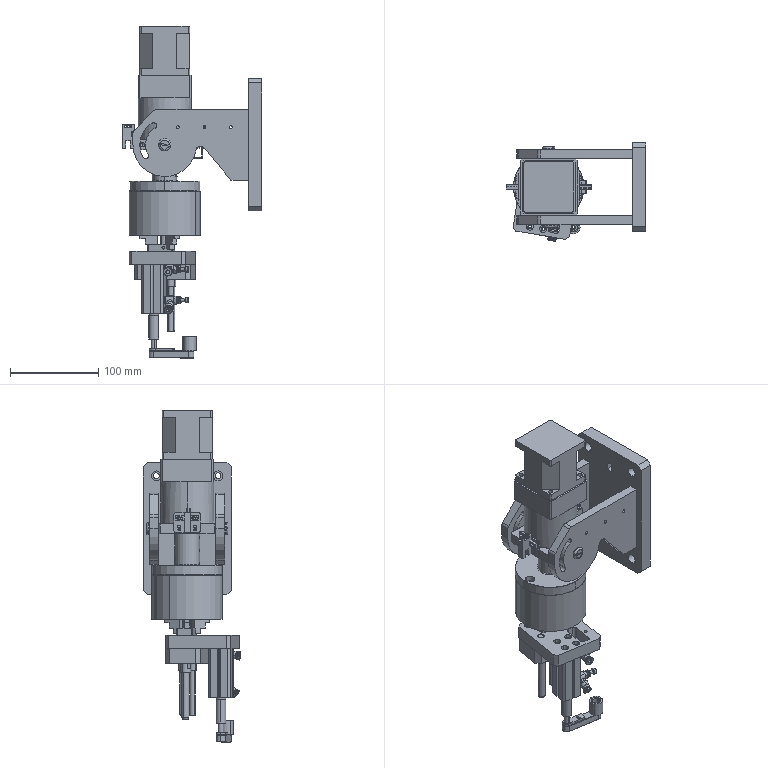Part | SolidWorks | 34 solids | 1429 faces | box 158.2 x 110.899 x 376 mm | volume 1286706 mm3 | plane 596 | cylinder 589 | cone 210 | spline 18 | torus 10 | sphere 6 | commonest cylinder face diameters 8 x54 3.3 x50 10 x37 5 x34 4 x28 6.5 x28